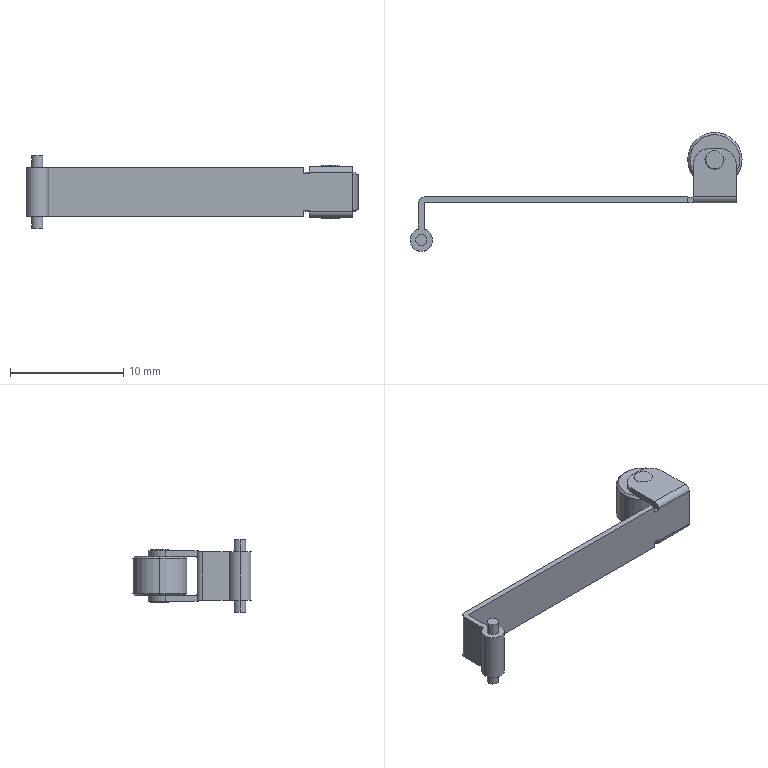Part | SolidWorks | features ICE 5, Fillet 3, Chamfer 2, Extrusion 1 | 3 solids | 53 faces | box 29.3 x 10.5 x 6.4 mm | volume 172.618 mm3 | plane 25 | cylinder 20 | cone 8 | commonest cylinder face diameters 1 x7 2 x5 3 x4 0.4 x2 4.8 x2
STEP:
#1=CARTESIAN_POINT('',(0.5,0.,3.2));
#2=VERTEX_POINT('',#1);
#3=CARTESIAN_POINT('',(-0.5,0.,3.2));
#4=VERTEX_POINT('',#3);
#5=CARTESIAN_POINT('',(0.,0.,3.2));
#6=DIRECTION('',(0.,0.,1.));
#7=DIRECTION('',(1.,0.,0.));
#8=AXIS2_PLACEMENT_3D('',#5,#6,#7);
#9=CIRCLE('',#8,0.5);
#10=EDGE_CURVE('',#2,#4,#9,.T.);
#11=ORIENTED_EDGE('',*,*,#10,.F.);
#12=CARTESIAN_POINT('',(0.5,0.,2.15));
#13=VERTEX_POINT('',#12);
#14=CARTESIAN_POINT('',(0.5,0.,3.2));
#15=DIRECTION('',(0.,0.,-1.));
#16=VECTOR('',#15,1000.);
#17=LINE('',#14,#16);
#18=EDGE_CURVE('',#2,#13,#17,.T.);
#19=ORIENTED_EDGE('',*,*,#18,.T.);
#20=CARTESIAN_POINT('',(-0.5,0.,2.15));
#21=VERTEX_POINT('',#20);
#22=CARTESIAN_POINT('',(0.,0.,2.15));
#23=DIRECTION('',(0.,0.,1.));
#24=DIRECTION('',(1.,0.,0.));
#25=AXIS2_PLACEMENT_3D('',#22,#23,#24);
#26=CIRCLE('',#25,0.5);
#27=EDGE_CURVE('',#13,#21,#26,.T.);
#28=ORIENTED_EDGE('',*,*,#27,.T.);
#29=CARTESIAN_POINT('',(-0.5,0.,3.2));
#30=DIRECTION('',(0.,0.,-1.));
#31=VECTOR('',#30,1000.);
#32=LINE('',#29,#31);
#33=EDGE_CURVE('',#4,#21,#32,.T.);
#34=ORIENTED_EDGE('',*,*,#33,.F.);
#35=EDGE_LOOP('',(#11,#19,#28,#34));
#36=FACE_OUTER_BOUND('',#35,.T.);
#37=CARTESIAN_POINT('',(0.,0.,3.2));
#38=DIRECTION('',(0.,0.,-1.));
#39=DIRECTION('',(-1.,0.,0.));
#40=AXIS2_PLACEMENT_3D('',#37,#38,#39);
#41=CYLINDRICAL_SURFACE('',#40,0.5);
#42=ADVANCED_FACE('',(#36),#41,.T.);
#43=CARTESIAN_POINT('',(-0.5,0.,-2.15));
#44=VERTEX_POINT('',#43);
#45=CARTESIAN_POINT('',(0.5,0.,-2.15));
#46=VERTEX_POINT('',#45);
#47=CARTESIAN_POINT('',(0.,0.,-2.15));
#48=DIRECTION('',(0.,0.,-1.));
#49=DIRECTION('',(1.,0.,0.));
#50=AXIS2_PLACEMENT_3D('',#47,#48,#49);
#51=CIRCLE('',#50,0.5);
#52=EDGE_CURVE('',#44,#46,#51,.T.);
#53=ORIENTED_EDGE('',*,*,#52,.T.);
#54=CARTESIAN_POINT('',(0.5,0.,-3.2));
#55=VERTEX_POINT('',#54);
#56=CARTESIAN_POINT('',(0.5,0.,3.2));
#57=DIRECTION('',(0.,0.,-1.));
#58=VECTOR('',#57,1000.);
#59=LINE('',#56,#58);
#60=EDGE_CURVE('',#46,#55,#59,.T.);
#61=ORIENTED_EDGE('',*,*,#60,.T.);
#62=CARTESIAN_POINT('',(-0.5,0.,-3.2));
#63=VERTEX_POINT('',#62);
#64=CARTESIAN_POINT('',(0.,0.,-3.2));
#65=DIRECTION('',(0.,0.,1.));
#66=DIRECTION('',(1.,0.,0.));
#67=AXIS2_PLACEMENT_3D('',#64,#65,#66);
#68=CIRCLE('',#67,0.5);
#69=EDGE_CURVE('',#55,#63,#68,.T.);
#70=ORIENTED_EDGE('',*,*,#69,.T.);
#71=CARTESIAN_POINT('',(-0.5,0.,3.2));
#72=DIRECTION('',(0.,0.,-1.));
#73=VECTOR('',#72,1000.);
#74=LINE('',#71,#73);
#75=EDGE_CURVE('',#44,#63,#74,.T.);
#76=ORIENTED_EDGE('',*,*,#75,.F.);
#77=EDGE_LOOP('',(#53,#61,#70,#76));
#78=FACE_OUTER_BOUND('',#77,.T.);
#79=CARTESIAN_POINT('',(0.,0.,3.2));
#80=DIRECTION('',(0.,0.,-1.));
#81=DIRECTION('',(-1.,0.,0.));
#82=AXIS2_PLACEMENT_3D('',#79,#80,#81);
#83=CYLINDRICAL_SURFACE('',#82,0.5);
#84=ADVANCED_FACE('',(#78),#83,.T.);
#85=CARTESIAN_POINT('',(1.,0.,2.15));
#86=VERTEX_POINT('',#85);
#87=CARTESIAN_POINT('',(0.25,0.9682,2.15));
#88=VERTEX_POINT('',#87);
#89=CARTESIAN_POINT('',(0.,0.,2.15));
#90=DIRECTION('',(0.,0.,1.));
#91=DIRECTION('',(1.,0.,0.));
#92=AXIS2_PLACEMENT_3D('',#89,#90,#91);
#93=CIRCLE('',#92,1.);
#94=EDGE_CURVE('',#86,#88,#93,.T.);
#95=ORIENTED_EDGE('',*,*,#94,.F.);
#96=CARTESIAN_POINT('',(1.,0.,-2.15));
#97=VERTEX_POINT('',#96);
#98=CARTESIAN_POINT('',(1.,0.,2.15));
#99=DIRECTION('',(0.,0.,-1.));
#100=VECTOR('',#99,1000.);
#101=LINE('',#98,#100);
#102=EDGE_CURVE('',#86,#97,#101,.T.);
#103=ORIENTED_EDGE('',*,*,#102,.T.);
#104=CARTESIAN_POINT('',(0.25,0.9682,-2.15));
#105=VERTEX_POINT('',#104);
#106=CARTESIAN_POINT('',(0.,0.,-2.15));
#107=DIRECTION('',(0.,0.,1.));
#108=DIRECTION('',(1.,0.,0.));
#109=AXIS2_PLACEMENT_3D('',#106,#107,#108);
#110=CIRCLE('',#109,1.);
#111=EDGE_CURVE('',#97,#105,#110,.T.);
#112=ORIENTED_EDGE('',*,*,#111,.T.);
#113=CARTESIAN_POINT('',(0.25,0.9682,2.15));
#114=DIRECTION('',(0.,0.,-1.));
#115=VECTOR('',#114,1000.);
#116=LINE('',#113,#115);
#117=EDGE_CURVE('',#88,#105,#116,.T.);
#118=ORIENTED_EDGE('',*,*,#117,.F.);
#119=EDGE_LOOP('',(#95,#103,#112,#118));
#120=FACE_OUTER_BOUND('',#119,.T.);
#121=CARTESIAN_POINT('',(0.,0.,2.15));
#122=DIRECTION('',(0.,0.,-1.));
#123=DIRECTION('',(-1.,0.,0.));
#124=AXIS2_PLACEMENT_3D('',#121,#122,#123);
#125=CYLINDRICAL_SURFACE('',#124,1.);
#126=ADVANCED_FACE('',(#120),#125,.T.);
#127=ORIENTED_EDGE('',*,*,#102,.F.);
#128=CARTESIAN_POINT('',(-1.,0.,2.15));
#129=VERTEX_POINT('',#128);
#130=CARTESIAN_POINT('',(0.,0.,2.15));
#131=DIRECTION('',(0.,0.,1.));
#132=DIRECTION('',(1.,0.,0.));
#133=AXIS2_PLACEMENT_3D('',#130,#131,#132);
#134=CIRCLE('',#133,1.);
#135=EDGE_CURVE('',#129,#86,#134,.T.);
#136=ORIENTED_EDGE('',*,*,#135,.F.);
#137=CARTESIAN_POINT('',(-1.,0.,-2.15));
#138=VERTEX_POINT('',#137);
#139=CARTESIAN_POINT('',(-1.,0.,2.15));
#140=DIRECTION('',(0.,0.,-1.));
#141=VECTOR('',#140,1000.);
#142=LINE('',#139,#141);
#143=EDGE_CURVE('',#129,#138,#142,.T.);
#144=ORIENTED_EDGE('',*,*,#143,.T.);
#145=CARTESIAN_POINT('',(0.,0.,-2.15));
#146=DIRECTION('',(0.,0.,1.));
#147=DIRECTION('',(1.,0.,0.));
#148=AXIS2_PLACEMENT_3D('',#145,#146,#147);
#149=CIRCLE('',#148,1.);
#150=EDGE_CURVE('',#138,#97,#149,.T.);
#151=ORIENTED_EDGE('',*,*,#150,.T.);
#152=EDGE_LOOP('',(#127,#136,#144,#151));
#153=FACE_OUTER_BOUND('',#152,.T.);
#154=CARTESIAN_POINT('',(0.,0.,2.15));
#155=DIRECTION('',(0.,0.,-1.));
#156=DIRECTION('',(-1.,0.,0.));
#157=AXIS2_PLACEMENT_3D('',#154,#155,#156);
#158=CYLINDRICAL_SURFACE('',#157,1.);
#159=ADVANCED_FACE('',(#153),#158,.T.);
#160=ORIENTED_EDGE('',*,*,#52,.F.);
#161=CARTESIAN_POINT('',(0.,0.,-2.15));
#162=DIRECTION('',(0.,0.,-1.));
#163=DIRECTION('',(1.,0.,0.));
#164=AXIS2_PLACEMENT_3D('',#161,#162,#163);
#165=CIRCLE('',#164,0.5);
#166=EDGE_CURVE('',#46,#44,#165,.T.);
#167=ORIENTED_EDGE('',*,*,#166,.F.);
#168=EDGE_LOOP('',(#160,#167));
#169=FACE_BOUND('',#168,.T.);
#170=CARTESIAN_POINT('',(23.5,3.8,-2.15));
#171=VERTEX_POINT('',#170);
#172=CARTESIAN_POINT('',(0.25,3.8,-2.15));
#173=VERTEX_POINT('',#172);
#174=CARTESIAN_POINT('',(0.25,3.8,-2.15));
#175=DIRECTION('',(-1.,0.,0.));
#176=VECTOR('',#175,1000.);
#177=LINE('',#174,#176);
#178=EDGE_CURVE('',#171,#173,#177,.T.);
#179=ORIENTED_EDGE('',*,*,#178,.F.);
#180=CARTESIAN_POINT('',(23.5,3.3,-2.15));
#181=VERTEX_POINT('',#180);
#182=CARTESIAN_POINT('',(23.5,0.,-2.15));
#183=DIRECTION('',(0.,-1.,0.));
#184=VECTOR('',#183,1000.);
#185=LINE('',#182,#184);
#186=EDGE_CURVE('',#171,#181,#185,.T.);
#187=ORIENTED_EDGE('',*,*,#186,.T.);
#188=CARTESIAN_POINT('',(0.25,3.3,-2.15));
#189=VERTEX_POINT('',#188);
#190=CARTESIAN_POINT('',(0.25,3.3,-2.15));
#191=DIRECTION('',(1.,0.,0.));
#192=VECTOR('',#191,1000.);
#193=LINE('',#190,#192);
#194=EDGE_CURVE('',#189,#181,#193,.T.);
#195=ORIENTED_EDGE('',*,*,#194,.F.);
#196=CARTESIAN_POINT('',(0.25,3.3,-2.15));
#197=DIRECTION('',(0.,1.,0.));
#198=VECTOR('',#197,1000.);
#199=LINE('',#196,#198);
#200=EDGE_CURVE('',#105,#189,#199,.T.);
#201=ORIENTED_EDGE('',*,*,#200,.F.);
#202=ORIENTED_EDGE('',*,*,#111,.F.);
#203=ORIENTED_EDGE('',*,*,#150,.F.);
#204=CARTESIAN_POINT('',(-0.25,0.9682,-2.15));
#205=VERTEX_POINT('',#204);
#206=CARTESIAN_POINT('',(0.,0.,-2.15));
#207=DIRECTION('',(0.,0.,1.));
#208=DIRECTION('',(1.,0.,0.));
#209=AXIS2_PLACEMENT_3D('',#206,#207,#208);
#210=CIRCLE('',#209,1.);
#211=EDGE_CURVE('',#205,#138,#210,.T.);
#212=ORIENTED_EDGE('',*,*,#211,.F.);
#213=CARTESIAN_POINT('',(-0.25,3.3,-2.15));
#214=VERTEX_POINT('',#213);
#215=CARTESIAN_POINT('',(-0.25,3.3,-2.15));
#216=DIRECTION('',(0.,-1.,0.));
#217=VECTOR('',#216,1000.);
#218=LINE('',#215,#217);
#219=EDGE_CURVE('',#214,#205,#218,.T.);
#220=ORIENTED_EDGE('',*,*,#219,.F.);
#221=CARTESIAN_POINT('',(0.25,3.3,-2.15));
#222=DIRECTION('',(0.,0.,1.));
#223=DIRECTION('',(-1.,0.,0.));
#224=AXIS2_PLACEMENT_3D('',#221,#222,#223);
#225=CIRCLE('',#224,0.5);
#226=EDGE_CURVE('',#173,#214,#225,.T.);
#227=ORIENTED_EDGE('',*,*,#226,.F.);
#228=EDGE_LOOP('',(#179,#187,#195,#201,#202,#203,#212,#220,#227));
#229=FACE_OUTER_BOUND('',#228,.T.);
#230=CARTESIAN_POINT('',(0.,0.,-2.15));
#231=DIRECTION('',(0.,0.,1.));
#232=DIRECTION('',(1.,0.,0.));
#233=AXIS2_PLACEMENT_3D('',#230,#231,#232);
#234=PLANE('',#233);
#235=ADVANCED_FACE('',(#169,#229),#234,.F.);
#236=CARTESIAN_POINT('',(23.5,3.8,2.15));
#237=VERTEX_POINT('',#236);
#238=CARTESIAN_POINT('',(23.5,3.3,2.15));
#239=VERTEX_POINT('',#238);
#240=CARTESIAN_POINT('',(23.5,0.,2.15));
#241=DIRECTION('',(0.,-1.,0.));
#242=VECTOR('',#241,1000.);
#243=LINE('',#240,#242);
#244=EDGE_CURVE('',#237,#239,#243,.T.);
#245=ORIENTED_EDGE('',*,*,#244,.F.);
#246=CARTESIAN_POINT('',(0.25,3.8,2.15));
#247=VERTEX_POINT('',#246);
#248=CARTESIAN_POINT('',(0.25,3.8,2.15));
#249=DIRECTION('',(-1.,0.,0.));
#250=VECTOR('',#249,1000.);
#251=LINE('',#248,#250);
#252=EDGE_CURVE('',#237,#247,#251,.T.);
#253=ORIENTED_EDGE('',*,*,#252,.T.);
#254=CARTESIAN_POINT('',(-0.25,3.3,2.15));
#255=VERTEX_POINT('',#254);
#256=CARTESIAN_POINT('',(0.25,3.3,2.15));
#257=DIRECTION('',(0.,0.,1.));
#258=DIRECTION('',(-1.,0.,0.));
#259=AXIS2_PLACEMENT_3D('',#256,#257,#258);
#260=CIRCLE('',#259,0.5);
#261=EDGE_CURVE('',#247,#255,#260,.T.);
#262=ORIENTED_EDGE('',*,*,#261,.T.);
#263=CARTESIAN_POINT('',(-0.25,0.9682,2.15));
#264=VERTEX_POINT('',#263);
#265=CARTESIAN_POINT('',(-0.25,3.3,2.15));
#266=DIRECTION('',(0.,-1.,0.));
#267=VECTOR('',#266,1000.);
#268=LINE('',#265,#267);
#269=EDGE_CURVE('',#255,#264,#268,.T.);
#270=ORIENTED_EDGE('',*,*,#269,.T.);
#271=CARTESIAN_POINT('',(0.,0.,2.15));
#272=DIRECTION('',(0.,0.,1.));
#273=DIRECTION('',(1.,0.,0.));
#274=AXIS2_PLACEMENT_3D('',#271,#272,#273);
#275=CIRCLE('',#274,1.);
#276=EDGE_CURVE('',#264,#129,#275,.T.);
#277=ORIENTED_EDGE('',*,*,#276,.T.);
#278=ORIENTED_EDGE('',*,*,#135,.T.);
#279=ORIENTED_EDGE('',*,*,#94,.T.);
#280=CARTESIAN_POINT('',(0.25,3.3,2.15));
#281=VERTEX_POINT('',#280);
#282=CARTESIAN_POINT('',(0.25,3.3,2.15));
#283=DIRECTION('',(0.,1.,0.));
#284=VECTOR('',#283,1000.);
#285=LINE('',#282,#284);
#286=EDGE_CURVE('',#88,#281,#285,.T.);
#287=ORIENTED_EDGE('',*,*,#286,.T.);
#288=CARTESIAN_POINT('',(0.25,3.3,2.15));
#289=DIRECTION('',(1.,0.,0.));
#290=VECTOR('',#289,1000.);
#291=LINE('',#288,#290);
#292=EDGE_CURVE('',#281,#239,#291,.T.);
#293=ORIENTED_EDGE('',*,*,#292,.T.);
#294=EDGE_LOOP('',(#245,#253,#262,#270,#277,#278,#279,#287,#293));
#295=FACE_OUTER_BOUND('',#294,.T.);
#296=CARTESIAN_POINT('',(0.,0.,2.15));
#297=DIRECTION('',(0.,0.,1.));
#298=DIRECTION('',(1.,0.,0.));
#299=AXIS2_PLACEMENT_3D('',#296,#297,#298);
#300=CIRCLE('',#299,0.5);
#301=EDGE_CURVE('',#21,#13,#300,.T.);
#302=ORIENTED_EDGE('',*,*,#301,.F.);
#303=ORIENTED_EDGE('',*,*,#27,.F.);
#304=EDGE_LOOP('',(#302,#303));
#305=FACE_BOUND('',#304,.T.);
#306=CARTESIAN_POINT('',(0.,0.,2.15));
#307=DIRECTION('',(0.,0.,1.));
#308=DIRECTION('',(1.,0.,0.));
#309=AXIS2_PLACEMENT_3D('',#306,#307,#308);
#310=PLANE('',#309);
#311=ADVANCED_FACE('',(#295,#305),#310,.T.);
#312=ORIENTED_EDGE('',*,*,#143,.F.);
#313=ORIENTED_EDGE('',*,*,#276,.F.);
#314=CARTESIAN_POINT('',(-0.25,0.9682,2.15));
#315=DIRECTION('',(0.,0.,-1.));
#316=VECTOR('',#315,1000.);
#317=LINE('',#314,#316);
#318=EDGE_CURVE('',#264,#205,#317,.T.);
#319=ORIENTED_EDGE('',*,*,#318,.T.);
#320=ORIENTED_EDGE('',*,*,#211,.T.);
#321=EDGE_LOOP('',(#312,#313,#319,#320));
#322=FACE_OUTER_BOUND('',#321,.T.);
#323=CARTESIAN_POINT('',(0.,0.,2.15));
#324=DIRECTION('',(0.,0.,-1.));
#325=DIRECTION('',(-1.,0.,0.));
#326=AXIS2_PLACEMENT_3D('',#323,#324,#325);
#327=CYLINDRICAL_SURFACE('',#326,1.);
#328=ADVANCED_FACE('',(#322),#327,.T.);
#329=ORIENTED_EDGE('',*,*,#200,.T.);
#330=CARTESIAN_POINT('',(0.25,3.3,2.15));
#331=DIRECTION('',(0.,0.,-1.));
#332=VECTOR('',#331,1000.);
#333=LINE('',#330,#332);
#334=EDGE_CURVE('',#281,#189,#333,.T.);
#335=ORIENTED_EDGE('',*,*,#334,.F.);
#336=ORIENTED_EDGE('',*,*,#286,.F.);
#337=ORIENTED_EDGE('',*,*,#117,.T.);
#338=EDGE_LOOP('',(#329,#335,#336,#337));
#339=FACE_OUTER_BOUND('',#338,.T.);
#340=CARTESIAN_POINT('',(0.25,3.3,2.15));
#341=DIRECTION('',(-1.,0.,0.));
#342=DIRECTION('',(0.,-1.,0.));
#343=AXIS2_PLACEMENT_3D('',#340,#341,#342);
#344=PLANE('',#343);
#345=ADVANCED_FACE('',(#339),#344,.F.);
#346=CARTESIAN_POINT('',(27.8,3.3,1.75));
#347=VERTEX_POINT('',#346);
#348=CARTESIAN_POINT('',(27.8,3.3,-1.75));
#349=VERTEX_POINT('',#348);
#350=CARTESIAN_POINT('',(27.8,3.3,2.15));
#351=DIRECTION('',(0.,0.,-1.));
#352=VECTOR('',#351,1000.);
#353=LINE('',#350,#352);
#354=EDGE_CURVE('',#347,#349,#353,.T.);
#355=ORIENTED_EDGE('',*,*,#354,.F.);
#356=CARTESIAN_POINT('',(24.,3.3,1.75));
#357=VERTEX_POINT('',#356);
#358=CARTESIAN_POINT('',(24.,3.3,1.75));
#359=DIRECTION('',(-1.,0.,0.));
#360=VECTOR('',#359,1000.);
#361=LINE('',#358,#360);
#362=EDGE_CURVE('',#347,#357,#361,.T.);
#363=ORIENTED_EDGE('',*,*,#362,.T.);
#364=CARTESIAN_POINT('',(24.,3.3,1.6));
#365=VERTEX_POINT('',#364);
#366=CARTESIAN_POINT('',(24.,3.3,2.15));
#367=DIRECTION('',(0.,0.,-1.));
#368=VECTOR('',#367,1000.);
#369=LINE('',#366,#368);
#370=EDGE_CURVE('',#357,#365,#369,.T.);
#371=ORIENTED_EDGE('',*,*,#370,.T.);
#372=CARTESIAN_POINT('',(23.5,3.3,1.6));
#373=VERTEX_POINT('',#372);
#374=CARTESIAN_POINT('',(0.25,3.3,1.6));
#375=DIRECTION('',(-1.,0.,0.));
#376=VECTOR('',#375,1000.);
#377=LINE('',#374,#376);
#378=EDGE_CURVE('',#365,#373,#377,.T.);
#379=ORIENTED_EDGE('',*,*,#378,.T.);
#380=CARTESIAN_POINT('',(23.5,3.3,2.15));
#381=DIRECTION('',(0.,0.,1.));
#382=VECTOR('',#381,1000.);
#383=LINE('',#380,#382);
#384=EDGE_CURVE('',#373,#239,#383,.T.);
#385=ORIENTED_EDGE('',*,*,#384,.T.);
#386=ORIENTED_EDGE('',*,*,#292,.F.);
#387=ORIENTED_EDGE('',*,*,#334,.T.);
#388=ORIENTED_EDGE('',*,*,#194,.T.);
#389=CARTESIAN_POINT('',(23.5,3.3,-1.6));
#390=VERTEX_POINT('',#389);
#391=CARTESIAN_POINT('',(23.5,3.3,2.15));
#392=DIRECTION('',(0.,0.,1.));
#393=VECTOR('',#392,1000.);
#394=LINE('',#391,#393);
#395=EDGE_CURVE('',#181,#390,#394,.T.);
#396=ORIENTED_EDGE('',*,*,#395,.T.);
#397=CARTESIAN_POINT('',(24.,3.3,-1.6));
#398=VERTEX_POINT('',#397);
#399=CARTESIAN_POINT('',(0.25,3.3,-1.6));
#400=DIRECTION('',(1.,0.,0.));
#401=VECTOR('',#400,1000.);
#402=LINE('',#399,#401);
#403=EDGE_CURVE('',#390,#398,#402,.T.);
#404=ORIENTED_EDGE('',*,*,#403,.T.);
#405=CARTESIAN_POINT('',(24.,3.3,-1.75));
#406=VERTEX_POINT('',#405);
#407=CARTESIAN_POINT('',(24.,3.3,-2.15));
#408=DIRECTION('',(0.,0.,-1.));
#409=VECTOR('',#408,1000.);
#410=LINE('',#407,#409);
#411=EDGE_CURVE('',#398,#406,#410,.T.);
#412=ORIENTED_EDGE('',*,*,#411,.T.);
#413=CARTESIAN_POINT('',(27.8,3.3,-1.75));
#414=DIRECTION('',(1.,0.,0.));
#415=VECTOR('',#414,1000.);
#416=LINE('',#413,#415);
#417=EDGE_CURVE('',#406,#349,#416,.T.);
#418=ORIENTED_EDGE('',*,*,#417,.T.);
#419=EDGE_LOOP('',(#355,#363,#371,#379,#385,#386,#387,#388,#396,#404,#412,#418));
#420=FACE_OUTER_BOUND('',#419,.T.);
#421=CARTESIAN_POINT('',(0.25,3.3,2.15));
#422=DIRECTION('',(0.,1.,0.));
#423=DIRECTION('',(0.,0.,1.));
#424=AXIS2_PLACEMENT_3D('',#421,#422,#423);
#425=PLANE('',#424);
#426=ADVANCED_FACE('',(#420),#425,.F.);
#427=CARTESIAN_POINT('',(27.8,3.8,-2.25));
#428=VERTEX_POINT('',#427);
#429=CARTESIAN_POINT('',(27.8,6.6,-2.25));
#430=VERTEX_POINT('',#429);
#431=CARTESIAN_POINT('',(27.8,3.3,-2.25));
#432=DIRECTION('',(0.,1.,0.));
#433=VECTOR('',#432,1000.);
#434=LINE('',#431,#433);
#435=EDGE_CURVE('',#428,#430,#434,.T.);
#436=ORIENTED_EDGE('',*,*,#435,.T.);
#437=CARTESIAN_POINT('',(27.8,6.6,-1.75));
#438=VERTEX_POINT('',#437);
#439=CARTESIAN_POINT('',(27.8,6.6,-1.75));
#440=DIRECTION('',(0.,0.,1.));
#441=VECTOR('',#440,1000.);
#442=LINE('',#439,#441);
#443=EDGE_CURVE('',#430,#438,#442,.T.);
#444=ORIENTED_EDGE('',*,*,#443,.T.);
#445=CARTESIAN_POINT('',(27.8,4.,-1.75));
#446=VERTEX_POINT('',#445);
#447=CARTESIAN_POINT('',(27.8,3.8,-1.75));
#448=DIRECTION('',(0.,-1.,0.));
#449=VECTOR('',#448,1000.);
#450=LINE('',#447,#449);
#451=EDGE_CURVE('',#438,#446,#450,.T.);
#452=ORIENTED_EDGE('',*,*,#451,.T.);
#453=CARTESIAN_POINT('',(27.8,3.8,-1.55));
#454=VERTEX_POINT('',#453);
#455=CARTESIAN_POINT('',(27.8,4.,-1.55));
#456=DIRECTION('',(-1.,0.,0.));
#457=DIRECTION('',(0.,0.,1.));
#458=AXIS2_PLACEMENT_3D('',#455,#456,#457);
#459=CIRCLE('',#458,0.2);
#460=EDGE_CURVE('',#446,#454,#459,.T.);
#461=ORIENTED_EDGE('',*,*,#460,.T.);
#462=CARTESIAN_POINT('',(27.8,3.8,1.55));
#463=VERTEX_POINT('',#462);
#464=CARTESIAN_POINT('',(27.8,3.8,2.15));
#465=DIRECTION('',(0.,0.,-1.));
#466=VECTOR('',#465,1000.);
#467=LINE('',#464,#466);
#468=EDGE_CURVE('',#463,#454,#467,.T.);
#469=ORIENTED_EDGE('',*,*,#468,.F.);
#470=CARTESIAN_POINT('',(27.8,4.,1.75));
#471=VERTEX_POINT('',#470);
#472=CARTESIAN_POINT('',(27.8,4.,1.55));
#473=DIRECTION('',(-1.,0.,0.));
#474=DIRECTION('',(0.,0.,1.));
#475=AXIS2_PLACEMENT_3D('',#472,#473,#474);
#476=CIRCLE('',#475,0.2);
#477=EDGE_CURVE('',#463,#471,#476,.T.);
#478=ORIENTED_EDGE('',*,*,#477,.T.);
#479=CARTESIAN_POINT('',(27.8,6.6,1.75));
#480=VERTEX_POINT('',#479);
#481=CARTESIAN_POINT('',(27.8,3.8,1.75));
#482=DIRECTION('',(0.,1.,0.));
#483=VECTOR('',#482,1000.);
#484=LINE('',#481,#483);
#485=EDGE_CURVE('',#471,#480,#484,.T.);
#486=ORIENTED_EDGE('',*,*,#485,.T.);
#487=CARTESIAN_POINT('',(27.8,6.6,2.25));
#488=VERTEX_POINT('',#487);
#489=CARTESIAN_POINT('',(27.8,6.6,2.25));
#490=DIRECTION('',(0.,0.,1.));
#491=VECTOR('',#490,1000.);
#492=LINE('',#489,#491);
#493=EDGE_CURVE('',#480,#488,#492,.T.);
#494=ORIENTED_EDGE('',*,*,#493,.T.);
#495=CARTESIAN_POINT('',(27.8,3.8,2.25));
#496=VERTEX_POINT('',#495);
#497=CARTESIAN_POINT('',(27.8,3.3,2.25));
#498=DIRECTION('',(0.,-1.,0.));
#499=VECTOR('',#498,1000.);
#500=LINE('',#497,#499);
#501=EDGE_CURVE('',#488,#496,#500,.T.);
#502=ORIENTED_EDGE('',*,*,#501,.T.);
#503=CARTESIAN_POINT('',(27.8,3.8,1.75));
#504=DIRECTION('',(1.,0.,0.));
#505=DIRECTION('',(0.,0.,1.));
#506=AXIS2_PLACEMENT_3D('',#503,#504,#505);
#507=CIRCLE('',#506,0.5);
#508=EDGE_CURVE('',#496,#347,#507,.T.);
#509=ORIENTED_EDGE('',*,*,#508,.T.);
#510=ORIENTED_EDGE('',*,*,#354,.T.);
#511=CARTESIAN_POINT('',(27.8,3.8,-1.75));
#512=DIRECTION('',(1.,0.,0.));
#513=DIRECTION('',(0.,0.,1.));
#514=AXIS2_PLACEMENT_3D('',#511,#512,#513);
#515=CIRCLE('',#514,0.5);
#516=EDGE_CURVE('',#349,#428,#515,.T.);
#517=ORIENTED_EDGE('',*,*,#516,.T.);
#518=EDGE_LOOP('',(#436,#444,#452,#461,#469,#478,#486,#494,#502,#509,#510,#517));
#519=FACE_OUTER_BOUND('',#518,.T.);
#520=CARTESIAN_POINT('',(27.8,3.8,2.15));
#521=DIRECTION('',(-1.,0.,0.));
#522=DIRECTION('',(0.,0.,1.));
#523=AXIS2_PLACEMENT_3D('',#520,#521,#522);
#524=PLANE('',#523);
#525=ADVANCED_FACE('',(#519),#524,.F.);
#526=ORIENTED_EDGE('',*,*,#252,.F.);
#527=CARTESIAN_POINT('',(23.5,3.8,1.6));
#528=VERTEX_POINT('',#527);
#529=CARTESIAN_POINT('',(23.5,3.8,2.25));
#530=DIRECTION('',(0.,0.,1.));
#531=VECTOR('',#530,1000.);
#532=LINE('',#529,#531);
#533=EDGE_CURVE('',#528,#237,#532,.T.);
#534=ORIENTED_EDGE('',*,*,#533,.F.);
#535=CARTESIAN_POINT('',(24.,3.8,1.6));
#536=VERTEX_POINT('',#535);
#537=CARTESIAN_POINT('',(24.,3.8,1.6));
#538=DIRECTION('',(-1.,0.,0.));
#539=VECTOR('',#538,1000.);
#540=LINE('',#537,#539);
#541=EDGE_CURVE('',#536,#528,#540,.T.);
#542=ORIENTED_EDGE('',*,*,#541,.F.);
#543=CARTESIAN_POINT('',(24.,3.8,1.55));
#544=VERTEX_POINT('',#543);
#545=CARTESIAN_POINT('',(24.,3.8,2.15));
#546=DIRECTION('',(0.,0.,-1.));
#547=VECTOR('',#546,1000.);
#548=LINE('',#545,#547);
#549=EDGE_CURVE('',#536,#544,#548,.T.);
#550=ORIENTED_EDGE('',*,*,#549,.T.);
#551=CARTESIAN_POINT('',(0.25,3.8,1.55));
#552=DIRECTION('',(1.,0.,0.));
#553=VECTOR('',#552,1000.);
#554=LINE('',#551,#553);
#555=EDGE_CURVE('',#544,#463,#554,.T.);
#556=ORIENTED_EDGE('',*,*,#555,.T.);
#557=ORIENTED_EDGE('',*,*,#468,.T.);
#558=CARTESIAN_POINT('',(24.,3.8,-1.55));
#559=VERTEX_POINT('',#558);
#560=CARTESIAN_POINT('',(0.25,3.8,-1.55));
#561=DIRECTION('',(-1.,0.,0.));
#562=VECTOR('',#561,1000.);
#563=LINE('',#560,#562);
#564=EDGE_CURVE('',#454,#559,#563,.T.);
#565=ORIENTED_EDGE('',*,*,#564,.T.);
#566=CARTESIAN_POINT('',(24.,3.8,-1.6));
#567=VERTEX_POINT('',#566);
#568=CARTESIAN_POINT('',(24.,3.8,-2.15));
#569=DIRECTION('',(0.,0.,-1.));
#570=VECTOR('',#569,1000.);
#571=LINE('',#568,#570);
#572=EDGE_CURVE('',#559,#567,#571,.T.);
#573=ORIENTED_EDGE('',*,*,#572,.T.);
#574=CARTESIAN_POINT('',(23.5,3.8,-1.6));
#575=VERTEX_POINT('',#574);
#576=CARTESIAN_POINT('',(24.,3.8,-1.6));
#577=DIRECTION('',(1.,0.,0.));
#578=VECTOR('',#577,1000.);
#579=LINE('',#576,#578);
#580=EDGE_CURVE('',#575,#567,#579,.T.);
#581=ORIENTED_EDGE('',*,*,#580,.F.);
#582=CARTESIAN_POINT('',(23.5,3.8,-2.25));
#583=DIRECTION('',(0.,0.,1.));
#584=VECTOR('',#583,1000.);
#585=LINE('',#582,#584);
#586=EDGE_CURVE('',#171,#575,#585,.T.);
#587=ORIENTED_EDGE('',*,*,#586,.F.);
#588=ORIENTED_EDGE('',*,*,#178,.T.);
#589=CARTESIAN_POINT('',(0.25,3.8,2.15));
#590=DIRECTION('',(0.,0.,-1.));
#591=VECTOR('',#590,1000.);
#592=LINE('',#589,#591);
#593=EDGE_CURVE('',#247,#173,#592,.T.);
#594=ORIENTED_EDGE('',*,*,#593,.F.);
#595=EDGE_LOOP('',(#526,#534,#542,#550,#556,#557,#565,#573,#581,#587,#588,#594));
#596=FACE_OUTER_BOUND('',#595,.T.);
#597=CARTESIAN_POINT('',(0.25,3.8,2.15));
#598=DIRECTION('',(0.,-1.,0.));
#599=DIRECTION('',(1.,0.,0.));
#600=AXIS2_PLACEMENT_3D('',#597,#598,#599);
#601=PLANE('',#600);
#602=ADVANCED_FACE('',(#596),#601,.F.);
#603=ORIENTED_EDGE('',*,*,#226,.T.);
#604=CARTESIAN_POINT('',(-0.25,3.3,2.15));
#605=DIRECTION('',(0.,0.,-1.));
#606=VECTOR('',#605,1000.);
#607=LINE('',#604,#606);
#608=EDGE_CURVE('',#255,#214,#607,.T.);
#609=ORIENTED_EDGE('',*,*,#608,.F.);
#610=ORIENTED_EDGE('',*,*,#261,.F.);
#611=ORIENTED_EDGE('',*,*,#593,.T.);
#612=EDGE_LOOP('',(#603,#609,#610,#611));
#613=FACE_OUTER_BOUND('',#612,.T.);
#614=CARTESIAN_POINT('',(0.25,3.3,2.15));
#615=DIRECTION('',(0.,0.,-1.));
#616=DIRECTION('',(-1.,0.,0.));
#617=AXIS2_PLACEMENT_3D('',#614,#615,#616);
#618=CYLINDRICAL_SURFACE('',#617,0.5);
#619=ADVANCED_FACE('',(#613),#618,.T.);
#620=ORIENTED_EDGE('',*,*,#219,.T.);
#621=ORIENTED_EDGE('',*,*,#318,.F.);
#622=ORIENTED_EDGE('',*,*,#269,.F.);
#623=ORIENTED_EDGE('',*,*,#608,.T.);
#624=EDGE_LOOP('',(#620,#621,#622,#623));
#625=FACE_OUTER_BOUND('',#624,.T.);
#626=CARTESIAN_POINT('',(-0.25,3.3,2.15));
#627=DIRECTION('',(1.,0.,0.));
#628=DIRECTION('',(0.,1.,0.));
#629=AXIS2_PLACEMENT_3D('',#626,#627,#628);
#630=PLANE('',#629);
#631=ADVANCED_FACE('',(#625),#630,.F.);
#632=CARTESIAN_POINT('',(0.,0.,-3.2));
#633=DIRECTION('',(0.,0.,1.));
#634=DIRECTION('',(1.,0.,0.));
#635=AXIS2_PLACEMENT_3D('',#632,#633,#634);
#636=CIRCLE('',#635,0.5);
#637=EDGE_CURVE('',#63,#55,#636,.T.);
#638=ORIENTED_EDGE('',*,*,#637,.F.);
#639=ORIENTED_EDGE('',*,*,#69,.F.);
#640=EDGE_LOOP('',(#638,#639));
#641=FACE_OUTER_BOUND('',#640,.T.);
#642=CARTESIAN_POINT('',(0.,0.,-3.2));
#643=DIRECTION('',(0.,0.,1.));
#644=DIRECTION('',(1.,0.,0.));
#645=AXIS2_PLACEMENT_3D('',#642,#643,#644);
#646=PLANE('',#645);
#647=ADVANCED_FACE('',(#641),#646,.F.);
#648=ORIENTED_EDGE('',*,*,#60,.F.);
#649=ORIENTED_EDGE('',*,*,#166,.T.);
#650=ORIENTED_EDGE('',*,*,#75,.T.);
#651=ORIENTED_EDGE('',*,*,#637,.T.);
#652=EDGE_LOOP('',(#648,#649,#650,#651));
#653=FACE_OUTER_BOUND('',#652,.T.);
#654=CARTESIAN_POINT('',(0.,0.,3.2));
#655=DIRECTION('',(0.,0.,-1.));
#656=DIRECTION('',(-1.,0.,0.));
#657=AXIS2_PLACEMENT_3D('',#654,#655,#656);
#658=CYLINDRICAL_SURFACE('',#657,0.5);
#659=ADVANCED_FACE('',(#653),#658,.T.);
#660=ORIENTED_EDGE('',*,*,#18,.F.);
#661=CARTESIAN_POINT('',(0.,0.,3.2));
#662=DIRECTION('',(0.,0.,1.));
#663=DIRECTION('',(1.,0.,0.));
#664=AXIS2_PLACEMENT_3D('',#661,#662,#663);
#665=CIRCLE('',#664,0.5);
#666=EDGE_CURVE('',#4,#2,#665,.T.);
#667=ORIENTED_EDGE('',*,*,#666,.F.);
#668=ORIENTED_EDGE('',*,*,#33,.T.);
#669=ORIENTED_EDGE('',*,*,#301,.T.);
#670=EDGE_LOOP('',(#660,#667,#668,#669));
#671=FACE_OUTER_BOUND('',#670,.T.);
#672=CARTESIAN_POINT('',(0.,0.,3.2));
#673=DIRECTION('',(0.,0.,-1.));
#674=DIRECTION('',(-1.,0.,0.));
#675=AXIS2_PLACEMENT_3D('',#672,#673,#674);
#676=CYLINDRICAL_SURFACE('',#675,0.5);
#677=ADVANCED_FACE('',(#671),#676,.T.);
#678=ORIENTED_EDGE('',*,*,#666,.T.);
#679=ORIENTED_EDGE('',*,*,#10,.T.);
#680=EDGE_LOOP('',(#678,#679));
#681=FACE_OUTER_BOUND('',#680,.T.);
#682=CARTESIAN_POINT('',(0.,0.,3.2));
#683=DIRECTION('',(0.,0.,1.));
#684=DIRECTION('',(1.,0.,0.));
#685=AXIS2_PLACEMENT_3D('',#682,#683,#684);
#686=PLANE('',#685);
#687=ADVANCED_FACE('',(#681),#686,.T.);
#688=ORIENTED_EDGE('',*,*,#451,.F.);
#689=CARTESIAN_POINT('',(26.3,8.1,-1.75));
#690=VERTEX_POINT('',#689);
#691=CARTESIAN_POINT('',(26.3,6.6,-1.75));
#692=DIRECTION('',(0.,0.,1.));
#693=DIRECTION('',(0.,-1.,0.));
#694=AXIS2_PLACEMENT_3D('',#691,#692,#693);
#695=CIRCLE('',#694,1.5);
#696=EDGE_CURVE('',#438,#690,#695,.T.);
#697=ORIENTED_EDGE('',*,*,#696,.T.);
#698=CARTESIAN_POINT('',(25.5,8.1,-1.75));
#699=VERTEX_POINT('',#698);
#700=CARTESIAN_POINT('',(24.,8.1,-1.75));
#701=DIRECTION('',(1.,0.,0.));
#702=VECTOR('',#701,1000.);
#703=LINE('',#700,#702);
#704=EDGE_CURVE('',#699,#690,#703,.T.);
#705=ORIENTED_EDGE('',*,*,#704,.F.);
#706=CARTESIAN_POINT('',(24.,6.6,-1.75));
#707=VERTEX_POINT('',#706);
#708=CARTESIAN_POINT('',(25.5,6.6,-1.75));
#709=DIRECTION('',(0.,0.,1.));
#710=DIRECTION('',(0.,-1.,0.));
#711=AXIS2_PLACEMENT_3D('',#708,#709,#710);
#712=CIRCLE('',#711,1.5);
#713=EDGE_CURVE('',#699,#707,#712,.T.);
#714=ORIENTED_EDGE('',*,*,#713,.T.);
#715=CARTESIAN_POINT('',(24.,4.,-1.75));
#716=VERTEX_POINT('',#715);
#717=CARTESIAN_POINT('',(24.,3.8,-1.75));
#718=DIRECTION('',(0.,-1.,0.));
#719=VECTOR('',#718,1000.);
#720=LINE('',#717,#719);
#721=EDGE_CURVE('',#707,#716,#720,.T.);
#722=ORIENTED_EDGE('',*,*,#721,.T.);
#723=CARTESIAN_POINT('',(24.,4.,-1.75));
#724=DIRECTION('',(1.,0.,0.));
#725=VECTOR('',#724,1000.);
#726=LINE('',#723,#725);
#727=EDGE_CURVE('',#716,#446,#726,.T.);
#728=ORIENTED_EDGE('',*,*,#727,.T.);
#729=EDGE_LOOP('',(#688,#697,#705,#714,#722,#728));
#730=FACE_OUTER_BOUND('',#729,.T.);
#731=CARTESIAN_POINT('',(24.,3.8,-1.75));
#732=DIRECTION('',(0.,0.,1.));
#733=DIRECTION('',(0.,-1.,0.));
#734=AXIS2_PLACEMENT_3D('',#731,#732,#733);
#735=PLANE('',#734);
#736=ADVANCED_FACE('',(#730),#735,.T.);
#737=ORIENTED_EDGE('',*,*,#704,.T.);
#738=CARTESIAN_POINT('',(26.3,8.1,-2.25));
#739=VERTEX_POINT('',#738);
#740=CARTESIAN_POINT('',(26.3,8.1,-2.25));
#741=DIRECTION('',(0.,0.,-1.));
#742=VECTOR('',#741,1000.);
#743=LINE('',#740,#742);
#744=EDGE_CURVE('',#690,#739,#743,.T.);
#745=ORIENTED_EDGE('',*,*,#744,.T.);
#746=CARTESIAN_POINT('',(25.5,8.1,-2.25));
#747=VERTEX_POINT('',#746);
#748=CARTESIAN_POINT('',(24.,8.1,-2.25));
#749=DIRECTION('',(1.,0.,0.));
#750=VECTOR('',#749,1000.);
#751=LINE('',#748,#750);
#752=EDGE_CURVE('',#747,#739,#751,.T.);
#753=ORIENTED_EDGE('',*,*,#752,.F.);
#754=CARTESIAN_POINT('',(25.5,8.1,-1.75));
#755=DIRECTION('',(0.,0.,1.));
#756=VECTOR('',#755,1000.);
#757=LINE('',#754,#756);
#758=EDGE_CURVE('',#747,#699,#757,.T.);
#759=ORIENTED_EDGE('',*,*,#758,.T.);
#760=EDGE_LOOP('',(#737,#745,#753,#759));
#761=FACE_OUTER_BOUND('',#760,.T.);
#762=CARTESIAN_POINT('',(24.,8.1,-2.25));
#763=DIRECTION('',(0.,1.,0.));
#764=DIRECTION('',(0.,0.,1.));
#765=AXIS2_PLACEMENT_3D('',#762,#763,#764);
#766=PLANE('',#765);
#767=ADVANCED_FACE('',(#761),#766,.T.);
#768=ORIENTED_EDGE('',*,*,#752,.T.);
#769=CARTESIAN_POINT('',(26.3,6.6,-2.25));
#770=DIRECTION('',(0.,0.,-1.));
#771=DIRECTION('',(0.,1.,0.));
#772=AXIS2_PLACEMENT_3D('',#769,#770,#771);
#773=CIRCLE('',#772,1.5);
#774=EDGE_CURVE('',#739,#430,#773,.T.);
#775=ORIENTED_EDGE('',*,*,#774,.T.);
#776=ORIENTED_EDGE('',*,*,#435,.F.);
#777=CARTESIAN_POINT('',(24.,3.8,-2.25));
#778=VERTEX_POINT('',#777);
#779=CARTESIAN_POINT('',(24.,3.8,-2.25));
#780=DIRECTION('',(-1.,0.,0.));
#781=VECTOR('',#780,1000.);
#782=LINE('',#779,#781);
#783=EDGE_CURVE('',#428,#778,#782,.T.);
#784=ORIENTED_EDGE('',*,*,#783,.T.);
#785=CARTESIAN_POINT('',(24.,6.6,-2.25));
#786=VERTEX_POINT('',#785);
#787=CARTESIAN_POINT('',(24.,3.3,-2.25));
#788=DIRECTION('',(0.,1.,0.));
#789=VECTOR('',#788,1000.);
#790=LINE('',#787,#789);
#791=EDGE_CURVE('',#778,#786,#790,.T.);
#792=ORIENTED_EDGE('',*,*,#791,.T.);
#793=CARTESIAN_POINT('',(25.5,6.6,-2.25));
#794=DIRECTION('',(0.,0.,-1.));
#795=DIRECTION('',(0.,1.,0.));
#796=AXIS2_PLACEMENT_3D('',#793,#794,#795);
#797=CIRCLE('',#796,1.5);
#798=EDGE_CURVE('',#786,#747,#797,.T.);
#799=ORIENTED_EDGE('',*,*,#798,.T.);
#800=EDGE_LOOP('',(#768,#775,#776,#784,#792,#799));
#801=FACE_OUTER_BOUND('',#800,.T.);
#802=CARTESIAN_POINT('',(24.,3.3,-2.25));
#803=DIRECTION('',(0.,0.,-1.));
#804=DIRECTION('',(0.,1.,0.));
#805=AXIS2_PLACEMENT_3D('',#802,#803,#804);
#806=PLANE('',#805);
#807=ADVANCED_FACE('',(#801),#806,.T.);
#808=ORIENTED_EDGE('',*,*,#721,.F.);
#809=CARTESIAN_POINT('',(24.,6.6,-2.25));
#810=DIRECTION('',(0.,0.,-1.));
#811=VECTOR('',#810,1000.);
#812=LINE('',#809,#811);
#813=EDGE_CURVE('',#707,#786,#812,.T.);
#814=ORIENTED_EDGE('',*,*,#813,.T.);
#815=ORIENTED_EDGE('',*,*,#791,.F.);
#816=CARTESIAN_POINT('',(24.,3.8,-1.75));
#817=DIRECTION('',(-1.,0.,0.));
#818=DIRECTION('',(0.,0.,-1.));
#819=AXIS2_PLACEMENT_3D('',#816,#817,#818);
#820=CIRCLE('',#819,0.5);
#821=EDGE_CURVE('',#778,#406,#820,.T.);
#822=ORIENTED_EDGE('',*,*,#821,.T.);
#823=ORIENTED_EDGE('',*,*,#411,.F.);
#824=CARTESIAN_POINT('',(24.,-1.,-1.6));
#825=DIRECTION('',(0.,1.,0.));
#826=VECTOR('',#825,1000.);
#827=LINE('',#824,#826);
#828=EDGE_CURVE('',#398,#567,#827,.T.);
#829=ORIENTED_EDGE('',*,*,#828,.T.);
#830=ORIENTED_EDGE('',*,*,#572,.F.);
#831=CARTESIAN_POINT('',(24.,4.,-1.55));
#832=DIRECTION('',(1.,0.,0.));
#833=DIRECTION('',(0.,0.,-1.));
#834=AXIS2_PLACEMENT_3D('',#831,#832,#833);
#835=CIRCLE('',#834,0.2);
#836=EDGE_CURVE('',#559,#716,#835,.T.);
#837=ORIENTED_EDGE('',*,*,#836,.T.);
#838=EDGE_LOOP('',(#808,#814,#815,#822,#823,#829,#830,#837));
#839=FACE_OUTER_BOUND('',#838,.T.);
#840=CARTESIAN_POINT('',(24.,3.3,-2.15));
#841=DIRECTION('',(1.,0.,0.));
#842=DIRECTION('',(0.,0.,-1.));
#843=AXIS2_PLACEMENT_3D('',#840,#841,#842);
#844=PLANE('',#843);
#845=ADVANCED_FACE('',(#839),#844,.F.);
#846=CARTESIAN_POINT('',(25.5,8.1,1.75));
#847=VERTEX_POINT('',#846);
#848=CARTESIAN_POINT('',(26.3,8.1,1.75));
#849=VERTEX_POINT('',#848);
#850=CARTESIAN_POINT('',(24.,8.1,1.75));
#851=DIRECTION('',(1.,0.,0.));
#852=VECTOR('',#851,1000.);
#853=LINE('',#850,#852);
#854=EDGE_CURVE('',#847,#849,#853,.T.);
#855=ORIENTED_EDGE('',*,*,#854,.T.);
#856=CARTESIAN_POINT('',(26.3,6.6,1.75));
#857=DIRECTION('',(0.,0.,-1.));
#858=DIRECTION('',(-1.,0.,0.));
#859=AXIS2_PLACEMENT_3D('',#856,#857,#858);
#860=CIRCLE('',#859,1.5);
#861=EDGE_CURVE('',#849,#480,#860,.T.);
#862=ORIENTED_EDGE('',*,*,#861,.T.);
#863=ORIENTED_EDGE('',*,*,#485,.F.);
#864=CARTESIAN_POINT('',(24.,4.,1.75));
#865=VERTEX_POINT('',#864);
#866=CARTESIAN_POINT('',(24.,4.,1.75));
#867=DIRECTION('',(-1.,0.,0.));
#868=VECTOR('',#867,1000.);
#869=LINE('',#866,#868);
#870=EDGE_CURVE('',#471,#865,#869,.T.);
#871=ORIENTED_EDGE('',*,*,#870,.T.);
#872=CARTESIAN_POINT('',(24.,6.6,1.75));
#873=VERTEX_POINT('',#872);
#874=CARTESIAN_POINT('',(24.,3.8,1.75));
#875=DIRECTION('',(0.,1.,0.));
#876=VECTOR('',#875,1000.);
#877=LINE('',#874,#876);
#878=EDGE_CURVE('',#865,#873,#877,.T.);
#879=ORIENTED_EDGE('',*,*,#878,.T.);
#880=CARTESIAN_POINT('',(25.5,6.6,1.75));
#881=DIRECTION('',(0.,0.,-1.));
#882=DIRECTION('',(-1.,0.,0.));
#883=AXIS2_PLACEMENT_3D('',#880,#881,#882);
#884=CIRCLE('',#883,1.5);
#885=EDGE_CURVE('',#873,#847,#884,.T.);
#886=ORIENTED_EDGE('',*,*,#885,.T.);
#887=EDGE_LOOP('',(#855,#862,#863,#871,#879,#886));
#888=FACE_OUTER_BOUND('',#887,.T.);
#889=CARTESIAN_POINT('',(24.,3.8,1.75));
#890=DIRECTION('',(0.,0.,-1.));
#891=DIRECTION('',(-1.,0.,0.));
#892=AXIS2_PLACEMENT_3D('',#889,#890,#891);
#893=PLANE('',#892);
#894=ADVANCED_FACE('',(#888),#893,.T.);
#895=ORIENTED_EDGE('',*,*,#501,.F.);
#896=CARTESIAN_POINT('',(26.3,8.1,2.25));
#897=VERTEX_POINT('',#896);
#898=CARTESIAN_POINT('',(26.3,6.6,2.25));
#899=DIRECTION('',(0.,0.,1.));
#900=DIRECTION('',(1.,0.,0.));
#901=AXIS2_PLACEMENT_3D('',#898,#899,#900);
#902=CIRCLE('',#901,1.5);
#903=EDGE_CURVE('',#488,#897,#902,.T.);
#904=ORIENTED_EDGE('',*,*,#903,.T.);
#905=CARTESIAN_POINT('',(25.5,8.1,2.25));
#906=VERTEX_POINT('',#905);
#907=CARTESIAN_POINT('',(24.,8.1,2.25));
#908=DIRECTION('',(1.,0.,0.));
#909=VECTOR('',#908,1000.);
#910=LINE('',#907,#909);
#911=EDGE_CURVE('',#906,#897,#910,.T.);
#912=ORIENTED_EDGE('',*,*,#911,.F.);
#913=CARTESIAN_POINT('',(24.,6.6,2.25));
#914=VERTEX_POINT('',#913);
#915=CARTESIAN_POINT('',(25.5,6.6,2.25));
#916=DIRECTION('',(0.,0.,1.));
#917=DIRECTION('',(1.,0.,0.));
#918=AXIS2_PLACEMENT_3D('',#915,#916,#917);
#919=CIRCLE('',#918,1.5);
#920=EDGE_CURVE('',#906,#914,#919,.T.);
#921=ORIENTED_EDGE('',*,*,#920,.T.);
#922=CARTESIAN_POINT('',(24.,3.8,2.25));
#923=VERTEX_POINT('',#922);
#924=CARTESIAN_POINT('',(24.,3.3,2.25));
#925=DIRECTION('',(0.,-1.,0.));
#926=VECTOR('',#925,1000.);
#927=LINE('',#924,#926);
#928=EDGE_CURVE('',#914,#923,#927,.T.);
#929=ORIENTED_EDGE('',*,*,#928,.T.);
#930=CARTESIAN_POINT('',(27.8,3.8,2.25));
#931=DIRECTION('',(1.,0.,0.));
#932=VECTOR('',#931,1000.);
#933=LINE('',#930,#932);
#934=EDGE_CURVE('',#923,#496,#933,.T.);
#935=ORIENTED_EDGE('',*,*,#934,.T.);
#936=EDGE_LOOP('',(#895,#904,#912,#921,#929,#935));
#937=FACE_OUTER_BOUND('',#936,.T.);
#938=CARTESIAN_POINT('',(24.,3.3,2.25));
#939=DIRECTION('',(0.,0.,1.));
#940=DIRECTION('',(1.,0.,0.));
#941=AXIS2_PLACEMENT_3D('',#938,#939,#940);
#942=PLANE('',#941);
#943=ADVANCED_FACE('',(#937),#942,.T.);
#944=ORIENTED_EDGE('',*,*,#911,.T.);
#945=CARTESIAN_POINT('',(26.3,8.1,1.75));
#946=DIRECTION('',(0.,0.,-1.));
#947=VECTOR('',#946,1000.);
#948=LINE('',#945,#947);
#949=EDGE_CURVE('',#897,#849,#948,.T.);
#950=ORIENTED_EDGE('',*,*,#949,.T.);
#951=ORIENTED_EDGE('',*,*,#854,.F.);
#952=CARTESIAN_POINT('',(25.5,8.1,2.25));
#953=DIRECTION('',(0.,0.,1.));
#954=VECTOR('',#953,1000.);
#955=LINE('',#952,#954);
#956=EDGE_CURVE('',#847,#906,#955,.T.);
#957=ORIENTED_EDGE('',*,*,#956,.T.);
#958=EDGE_LOOP('',(#944,#950,#951,#957));
#959=FACE_OUTER_BOUND('',#958,.T.);
#960=CARTESIAN_POINT('',(24.,8.1,2.25));
#961=DIRECTION('',(0.,1.,0.));
#962=DIRECTION('',(0.,0.,1.));
#963=AXIS2_PLACEMENT_3D('',#960,#961,#962);
#964=PLANE('',#963);
#965=ADVANCED_FACE('',(#959),#964,.T.);
#966=ORIENTED_EDGE('',*,*,#928,.F.);
#967=CARTESIAN_POINT('',(24.,6.6,1.75));
#968=DIRECTION('',(0.,0.,-1.));
#969=VECTOR('',#968,1000.);
#970=LINE('',#967,#969);
#971=EDGE_CURVE('',#914,#873,#970,.T.);
#972=ORIENTED_EDGE('',*,*,#971,.T.);
#973=ORIENTED_EDGE('',*,*,#878,.F.);
#974=CARTESIAN_POINT('',(24.,4.,1.55));
#975=DIRECTION('',(1.,0.,0.));
#976=DIRECTION('',(0.,0.,1.));
#977=AXIS2_PLACEMENT_3D('',#974,#975,#976);
#978=CIRCLE('',#977,0.2);
#979=EDGE_CURVE('',#865,#544,#978,.T.);
#980=ORIENTED_EDGE('',*,*,#979,.T.);
#981=ORIENTED_EDGE('',*,*,#549,.F.);
#982=CARTESIAN_POINT('',(24.,-1.,1.6));
#983=DIRECTION('',(0.,1.,0.));
#984=VECTOR('',#983,1000.);
#985=LINE('',#982,#984);
#986=EDGE_CURVE('',#365,#536,#985,.T.);
#987=ORIENTED_EDGE('',*,*,#986,.F.);
#988=ORIENTED_EDGE('',*,*,#370,.F.);
#989=CARTESIAN_POINT('',(24.,3.8,1.75));
#990=DIRECTION('',(-1.,0.,0.));
#991=DIRECTION('',(0.,0.,1.));
#992=AXIS2_PLACEMENT_3D('',#989,#990,#991);
#993=CIRCLE('',#992,0.5);
#994=EDGE_CURVE('',#357,#923,#993,.T.);
#995=ORIENTED_EDGE('',*,*,#994,.T.);
#996=EDGE_LOOP('',(#966,#972,#973,#980,#981,#987,#988,#995));
#997=FACE_OUTER_BOUND('',#996,.T.);
#998=CARTESIAN_POINT('',(24.,8.1,1.75));
#999=DIRECTION('',(-1.,0.,0.));
#1000=DIRECTION('',(0.,0.,1.));
#1001=AXIS2_PLACEMENT_3D('',#998,#999,#1000);
#1002=PLANE('',#1001);
#1003=ADVANCED_FACE('',(#997),#1002,.T.);
#1004=ORIENTED_EDGE('',*,*,#836,.F.);
#1005=ORIENTED_EDGE('',*,*,#564,.F.);
#1006=ORIENTED_EDGE('',*,*,#460,.F.);
#1007=ORIENTED_EDGE('',*,*,#727,.F.);
#1008=EDGE_LOOP('',(#1004,#1005,#1006,#1007));
#1009=FACE_OUTER_BOUND('',#1008,.T.);
#1010=CARTESIAN_POINT('',(24.,4.,-1.55));
#1011=DIRECTION('',(1.,0.,0.));
#1012=DIRECTION('',(0.,1.,0.));
#1013=AXIS2_PLACEMENT_3D('',#1010,#1011,#1012);
#1014=CYLINDRICAL_SURFACE('',#1013,0.2);
#1015=ADVANCED_FACE('',(#1009),#1014,.F.);
#1016=ORIENTED_EDGE('',*,*,#979,.F.);
#1017=ORIENTED_EDGE('',*,*,#870,.F.);
#1018=ORIENTED_EDGE('',*,*,#477,.F.);
#1019=ORIENTED_EDGE('',*,*,#555,.F.);
#1020=EDGE_LOOP('',(#1016,#1017,#1018,#1019));
#1021=FACE_OUTER_BOUND('',#1020,.T.);
#1022=CARTESIAN_POINT('',(0.25,4.,1.55));
#1023=DIRECTION('',(1.,0.,0.));
#1024=DIRECTION('',(0.,1.,0.));
#1025=AXIS2_PLACEMENT_3D('',#1022,#1023,#1024);
#1026=CYLINDRICAL_SURFACE('',#1025,0.2);
#1027=ADVANCED_FACE('',(#1021),#1026,.F.);
#1028=ORIENTED_EDGE('',*,*,#586,.T.);
#1029=CARTESIAN_POINT('',(23.5,-1.,-1.6));
#1030=DIRECTION('',(0.,1.,0.));
#1031=VECTOR('',#1030,1000.);
#1032=LINE('',#1029,#1031);
#1033=EDGE_CURVE('',#390,#575,#1032,.T.);
#1034=ORIENTED_EDGE('',*,*,#1033,.F.);
#1035=ORIENTED_EDGE('',*,*,#395,.F.);
#1036=ORIENTED_EDGE('',*,*,#186,.F.);
#1037=EDGE_LOOP('',(#1028,#1034,#1035,#1036));
#1038=FACE_OUTER_BOUND('',#1037,.T.);
#1039=CARTESIAN_POINT('',(23.5,-1.,-2.25));
#1040=DIRECTION('',(-1.,0.,0.));
#1041=DIRECTION('',(0.,0.,1.));
#1042=AXIS2_PLACEMENT_3D('',#1039,#1040,#1041);
#1043=PLANE('',#1042);
#1044=ADVANCED_FACE('',(#1038),#1043,.F.);
#1045=ORIENTED_EDGE('',*,*,#1033,.T.);
#1046=ORIENTED_EDGE('',*,*,#580,.T.);
#1047=ORIENTED_EDGE('',*,*,#828,.F.);
#1048=ORIENTED_EDGE('',*,*,#403,.F.);
#1049=EDGE_LOOP('',(#1045,#1046,#1047,#1048));
#1050=FACE_OUTER_BOUND('',#1049,.T.);
#1051=CARTESIAN_POINT('',(24.,-1.,-1.6));
#1052=DIRECTION('',(0.,0.,1.));
#1053=DIRECTION('',(1.,0.,0.));
#1054=AXIS2_PLACEMENT_3D('',#1051,#1052,#1053);
#1055=PLANE('',#1054);
#1056=ADVANCED_FACE('',(#1050),#1055,.F.);
#1057=ORIENTED_EDGE('',*,*,#986,.T.);
#1058=ORIENTED_EDGE('',*,*,#541,.T.);
#1059=CARTESIAN_POINT('',(23.5,-1.,1.6));
#1060=DIRECTION('',(0.,1.,0.));
#1061=VECTOR('',#1060,1000.);
#1062=LINE('',#1059,#1061);
#1063=EDGE_CURVE('',#373,#528,#1062,.T.);
#1064=ORIENTED_EDGE('',*,*,#1063,.F.);
#1065=ORIENTED_EDGE('',*,*,#378,.F.);
#1066=EDGE_LOOP('',(#1057,#1058,#1064,#1065));
#1067=FACE_OUTER_BOUND('',#1066,.T.);
#1068=CARTESIAN_POINT('',(24.,-1.,1.6));
#1069=DIRECTION('',(0.,0.,-1.));
#1070=DIRECTION('',(-1.,0.,0.));
#1071=AXIS2_PLACEMENT_3D('',#1068,#1069,#1070);
#1072=PLANE('',#1071);
#1073=ADVANCED_FACE('',(#1067),#1072,.F.);
#1074=ORIENTED_EDGE('',*,*,#244,.T.);
#1075=ORIENTED_EDGE('',*,*,#384,.F.);
#1076=ORIENTED_EDGE('',*,*,#1063,.T.);
#1077=ORIENTED_EDGE('',*,*,#533,.T.);
#1078=EDGE_LOOP('',(#1074,#1075,#1076,#1077));
#1079=FACE_OUTER_BOUND('',#1078,.T.);
#1080=CARTESIAN_POINT('',(23.5,-1.,2.25));
#1081=DIRECTION('',(-1.,0.,0.));
#1082=DIRECTION('',(0.,0.,1.));
#1083=AXIS2_PLACEMENT_3D('',#1080,#1081,#1082);
#1084=PLANE('',#1083);
#1085=ADVANCED_FACE('',(#1079),#1084,.F.);
#1086=ORIENTED_EDGE('',*,*,#994,.F.);
#1087=ORIENTED_EDGE('',*,*,#362,.F.);
#1088=ORIENTED_EDGE('',*,*,#508,.F.);
#1089=ORIENTED_EDGE('',*,*,#934,.F.);
#1090=EDGE_LOOP('',(#1086,#1087,#1088,#1089));
#1091=FACE_OUTER_BOUND('',#1090,.T.);
#1092=CARTESIAN_POINT('',(24.,3.8,1.75));
#1093=DIRECTION('',(-1.,0.,0.));
#1094=DIRECTION('',(0.,0.,1.));
#1095=AXIS2_PLACEMENT_3D('',#1092,#1093,#1094);
#1096=CYLINDRICAL_SURFACE('',#1095,0.5);
#1097=ADVANCED_FACE('',(#1091),#1096,.T.);
#1098=ORIENTED_EDGE('',*,*,#821,.F.);
#1099=ORIENTED_EDGE('',*,*,#783,.F.);
#1100=ORIENTED_EDGE('',*,*,#516,.F.);
#1101=ORIENTED_EDGE('',*,*,#417,.F.);
#1102=EDGE_LOOP('',(#1098,#1099,#1100,#1101));
#1103=FACE_OUTER_BOUND('',#1102,.T.);
#1104=CARTESIAN_POINT('',(0.25,3.8,-1.75));
#1105=DIRECTION('',(-1.,0.,0.));
#1106=DIRECTION('',(0.,0.,1.));
#1107=AXIS2_PLACEMENT_3D('',#1104,#1105,#1106);
#1108=CYLINDRICAL_SURFACE('',#1107,0.5);
#1109=ADVANCED_FACE('',(#1103),#1108,.T.);
#1110=ORIENTED_EDGE('',*,*,#774,.F.);
#1111=ORIENTED_EDGE('',*,*,#744,.F.);
#1112=ORIENTED_EDGE('',*,*,#696,.F.);
#1113=ORIENTED_EDGE('',*,*,#443,.F.);
#1114=EDGE_LOOP('',(#1110,#1111,#1112,#1113));
#1115=FACE_OUTER_BOUND('',#1114,.T.);
#1116=CARTESIAN_POINT('',(26.3,6.6,2.15));
#1117=DIRECTION('',(0.,0.,-1.));
#1118=DIRECTION('',(-1.,0.,0.));
#1119=AXIS2_PLACEMENT_3D('',#1116,#1117,#1118);
#1120=CYLINDRICAL_SURFACE('',#1119,1.5);
#1121=ADVANCED_FACE('',(#1115),#1120,.T.);
#1122=ORIENTED_EDGE('',*,*,#798,.F.);
#1123=ORIENTED_EDGE('',*,*,#813,.F.);
#1124=ORIENTED_EDGE('',*,*,#713,.F.);
#1125=ORIENTED_EDGE('',*,*,#758,.F.);
#1126=EDGE_LOOP('',(#1122,#1123,#1124,#1125));
#1127=FACE_OUTER_BOUND('',#1126,.T.);
#1128=CARTESIAN_POINT('',(25.5,6.6,-2.25));
#1129=DIRECTION('',(0.,0.,-1.));
#1130=DIRECTION('',(-1.,0.,0.));
#1131=AXIS2_PLACEMENT_3D('',#1128,#1129,#1130);
#1132=CYLINDRICAL_SURFACE('',#1131,1.5);
#1133=ADVANCED_FACE('',(#1127),#1132,.T.);
#1134=ORIENTED_EDGE('',*,*,#861,.F.);
#1135=ORIENTED_EDGE('',*,*,#949,.F.);
#1136=ORIENTED_EDGE('',*,*,#903,.F.);
#1137=ORIENTED_EDGE('',*,*,#493,.F.);
#1138=EDGE_LOOP('',(#1134,#1135,#1136,#1137));
#1139=FACE_OUTER_BOUND('',#1138,.T.);
#1140=CARTESIAN_POINT('',(26.3,6.6,2.15));
#1141=DIRECTION('',(0.,0.,-1.));
#1142=DIRECTION('',(-1.,0.,0.));
#1143=AXIS2_PLACEMENT_3D('',#1140,#1141,#1142);
#1144=CYLINDRICAL_SURFACE('',#1143,1.5);
#1145=ADVANCED_FACE('',(#1139),#1144,.T.);
#1146=ORIENTED_EDGE('',*,*,#885,.F.);
#1147=ORIENTED_EDGE('',*,*,#971,.F.);
#1148=ORIENTED_EDGE('',*,*,#920,.F.);
#1149=ORIENTED_EDGE('',*,*,#956,.F.);
#1150=EDGE_LOOP('',(#1146,#1147,#1148,#1149));
#1151=FACE_OUTER_BOUND('',#1150,.T.);
#1152=CARTESIAN_POINT('',(25.5,6.6,2.25));
#1153=DIRECTION('',(0.,0.,1.));
#1154=DIRECTION('',(1.,0.,0.));
#1155=AXIS2_PLACEMENT_3D('',#1152,#1153,#1154);
#1156=CYLINDRICAL_SURFACE('',#1155,1.5);
#1157=ADVANCED_FACE('',(#1151),#1156,.T.);
#1158=CLOSED_SHELL('',(#42,#84,#126,#159,#235,#311,#328,#345,#426,#525,#602,#619,#631,#647,#659,#677,#687,#736,#767,#807,#845,#894,#943,#965,#1003,#1015,#1027,#1044,#1056,#1073,#1085,#1097,#1109,#1121,#1133,#1145,#1157));
#1159=MANIFOLD_SOLID_BREP('',#1158);
#1160=CARTESIAN_POINT('',(25.1,7.1,-2.35));
#1161=VERTEX_POINT('',#1160);
#1162=CARTESIAN_POINT('',(26.7,7.1,-2.35));
#1163=VERTEX_POINT('',#1162);
#1164=CARTESIAN_POINT('',(25.9,7.1,-2.35));
#1165=DIRECTION('',(0.,0.,-1.));
#1166=DIRECTION('',(1.,0.,0.));
#1167=AXIS2_PLACEMENT_3D('',#1164,#1165,#1166);
#1168=CIRCLE('',#1167,0.8);
#1169=EDGE_CURVE('',#1161,#1163,#1168,.T.);
#1170=ORIENTED_EDGE('',*,*,#1169,.F.);
#1171=CARTESIAN_POINT('',(24.9,7.1,-2.15));
#1172=VERTEX_POINT('',#1171);
#1173=CARTESIAN_POINT('',(24.9,7.1,-2.15));
#1174=DIRECTION('',(-0.7071,0.,0.7071));
#1175=VECTOR('',#1174,1000.);
#1176=LINE('',#1173,#1175);
#1177=EDGE_CURVE('',#1161,#1172,#1176,.T.);
#1178=ORIENTED_EDGE('',*,*,#1177,.T.);
#1179=CARTESIAN_POINT('',(26.9,7.1,-2.15));
#1180=VERTEX_POINT('',#1179);
#1181=CARTESIAN_POINT('',(25.9,7.1,-2.15));
#1182=DIRECTION('',(0.,0.,1.));
#1183=DIRECTION('',(1.,0.,0.));
#1184=AXIS2_PLACEMENT_3D('',#1181,#1182,#1183);
#1185=CIRCLE('',#1184,1.);
#1186=EDGE_CURVE('',#1180,#1172,#1185,.T.);
#1187=ORIENTED_EDGE('',*,*,#1186,.F.);
#1188=CARTESIAN_POINT('',(26.9,7.1,-2.15));
#1189=DIRECTION('',(0.7071,0.,0.7071));
#1190=VECTOR('',#1189,1000.);
#1191=LINE('',#1188,#1190);
#1192=EDGE_CURVE('',#1163,#1180,#1191,.T.);
#1193=ORIENTED_EDGE('',*,*,#1192,.F.);
#1194=EDGE_LOOP('',(#1170,#1178,#1187,#1193));
#1195=FACE_OUTER_BOUND('',#1194,.T.);
#1196=CARTESIAN_POINT('',(25.9,7.1,-2.15));
#1197=DIRECTION('',(0.,0.,1.));
#1198=DIRECTION('',(1.,0.,0.));
#1199=AXIS2_PLACEMENT_3D('',#1196,#1197,#1198);
#1200=CONICAL_SURFACE('',#1199,1.,0.7854);
#1201=ADVANCED_FACE('',(#1195),#1200,.T.);
#1202=CARTESIAN_POINT('',(26.7,7.1,2.35));
#1203=VERTEX_POINT('',#1202);
#1204=CARTESIAN_POINT('',(25.1,7.1,2.35));
#1205=VERTEX_POINT('',#1204);
#1206=CARTESIAN_POINT('',(25.9,7.1,2.35));
#1207=DIRECTION('',(0.,0.,1.));
#1208=DIRECTION('',(1.,0.,0.));
#1209=AXIS2_PLACEMENT_3D('',#1206,#1207,#1208);
#1210=CIRCLE('',#1209,0.8);
#1211=EDGE_CURVE('',#1203,#1205,#1210,.T.);
#1212=ORIENTED_EDGE('',*,*,#1211,.F.);
#1213=CARTESIAN_POINT('',(26.9,7.1,2.15));
#1214=VERTEX_POINT('',#1213);
#1215=CARTESIAN_POINT('',(26.7,7.1,2.35));
#1216=DIRECTION('',(0.7071,0.,-0.7071));
#1217=VECTOR('',#1216,1000.);
#1218=LINE('',#1215,#1217);
#1219=EDGE_CURVE('',#1203,#1214,#1218,.T.);
#1220=ORIENTED_EDGE('',*,*,#1219,.T.);
#1221=CARTESIAN_POINT('',(24.9,7.1,2.15));
#1222=VERTEX_POINT('',#1221);
#1223=CARTESIAN_POINT('',(25.9,7.1,2.15));
#1224=DIRECTION('',(0.,0.,-1.));
#1225=DIRECTION('',(1.,0.,0.));
#1226=AXIS2_PLACEMENT_3D('',#1223,#1224,#1225);
#1227=CIRCLE('',#1226,1.);
#1228=EDGE_CURVE('',#1222,#1214,#1227,.T.);
#1229=ORIENTED_EDGE('',*,*,#1228,.F.);
#1230=CARTESIAN_POINT('',(25.1,7.1,2.35));
#1231=DIRECTION('',(-0.7071,0.,-0.7071));
#1232=VECTOR('',#1231,1000.);
#1233=LINE('',#1230,#1232);
#1234=EDGE_CURVE('',#1205,#1222,#1233,.T.);
#1235=ORIENTED_EDGE('',*,*,#1234,.F.);
#1236=EDGE_LOOP('',(#1212,#1220,#1229,#1235));
#1237=FACE_OUTER_BOUND('',#1236,.T.);
#1238=CARTESIAN_POINT('',(25.9,7.1,2.35));
#1239=DIRECTION('',(0.,0.,-1.));
#1240=DIRECTION('',(-1.,0.,0.));
#1241=AXIS2_PLACEMENT_3D('',#1238,#1239,#1240);
#1242=CONICAL_SURFACE('',#1241,0.8,0.7854);
#1243=ADVANCED_FACE('',(#1237),#1242,.T.);
#1244=ORIENTED_EDGE('',*,*,#1228,.T.);
#1245=CARTESIAN_POINT('',(26.9,7.1,2.35));
#1246=DIRECTION('',(0.,0.,-1.));
#1247=VECTOR('',#1246,1000.);
#1248=LINE('',#1245,#1247);
#1249=EDGE_CURVE('',#1214,#1180,#1248,.T.);
#1250=ORIENTED_EDGE('',*,*,#1249,.T.);
#1251=ORIENTED_EDGE('',*,*,#1186,.T.);
#1252=CARTESIAN_POINT('',(24.9,7.1,2.35));
#1253=DIRECTION('',(0.,0.,-1.));
#1254=VECTOR('',#1253,1000.);
#1255=LINE('',#1252,#1254);
#1256=EDGE_CURVE('',#1222,#1172,#1255,.T.);
#1257=ORIENTED_EDGE('',*,*,#1256,.F.);
#1258=EDGE_LOOP('',(#1244,#1250,#1251,#1257));
#1259=FACE_OUTER_BOUND('',#1258,.T.);
#1260=CARTESIAN_POINT('',(25.9,7.1,2.35));
#1261=DIRECTION('',(0.,0.,-1.));
#1262=DIRECTION('',(-1.,0.,0.));
#1263=AXIS2_PLACEMENT_3D('',#1260,#1261,#1262);
#1264=CYLINDRICAL_SURFACE('',#1263,1.);
#1265=ADVANCED_FACE('',(#1259),#1264,.T.);
#1266=ORIENTED_EDGE('',*,*,#1249,.F.);
#1267=CARTESIAN_POINT('',(25.9,7.1,2.15));
#1268=DIRECTION('',(0.,0.,-1.));
#1269=DIRECTION('',(1.,0.,0.));
#1270=AXIS2_PLACEMENT_3D('',#1267,#1268,#1269);
#1271=CIRCLE('',#1270,1.);
#1272=EDGE_CURVE('',#1214,#1222,#1271,.T.);
#1273=ORIENTED_EDGE('',*,*,#1272,.T.);
#1274=ORIENTED_EDGE('',*,*,#1256,.T.);
#1275=CARTESIAN_POINT('',(25.9,7.1,-2.15));
#1276=DIRECTION('',(0.,0.,1.));
#1277=DIRECTION('',(1.,0.,0.));
#1278=AXIS2_PLACEMENT_3D('',#1275,#1276,#1277);
#1279=CIRCLE('',#1278,1.);
#1280=EDGE_CURVE('',#1172,#1180,#1279,.T.);
#1281=ORIENTED_EDGE('',*,*,#1280,.T.);
#1282=EDGE_LOOP('',(#1266,#1273,#1274,#1281));
#1283=FACE_OUTER_BOUND('',#1282,.T.);
#1284=CARTESIAN_POINT('',(25.9,7.1,2.35));
#1285=DIRECTION('',(0.,0.,-1.));
#1286=DIRECTION('',(-1.,0.,0.));
#1287=AXIS2_PLACEMENT_3D('',#1284,#1285,#1286);
#1288=CYLINDRICAL_SURFACE('',#1287,1.);
#1289=ADVANCED_FACE('',(#1283),#1288,.T.);
#1290=CARTESIAN_POINT('',(25.9,7.1,2.35));
#1291=DIRECTION('',(0.,0.,1.));
#1292=DIRECTION('',(1.,0.,0.));
#1293=AXIS2_PLACEMENT_3D('',#1290,#1291,#1292);
#1294=CIRCLE('',#1293,0.8);
#1295=EDGE_CURVE('',#1205,#1203,#1294,.T.);
#1296=ORIENTED_EDGE('',*,*,#1295,.T.);
#1297=ORIENTED_EDGE('',*,*,#1211,.T.);
#1298=EDGE_LOOP('',(#1296,#1297));
#1299=FACE_OUTER_BOUND('',#1298,.T.);
#1300=CARTESIAN_POINT('',(25.9,7.1,2.35));
#1301=DIRECTION('',(0.,0.,1.));
#1302=DIRECTION('',(1.,0.,0.));
#1303=AXIS2_PLACEMENT_3D('',#1300,#1301,#1302);
#1304=PLANE('',#1303);
#1305=ADVANCED_FACE('',(#1299),#1304,.T.);
#1306=CARTESIAN_POINT('',(25.9,7.1,-2.35));
#1307=DIRECTION('',(0.,0.,-1.));
#1308=DIRECTION('',(1.,0.,0.));
#1309=AXIS2_PLACEMENT_3D('',#1306,#1307,#1308);
#1310=CIRCLE('',#1309,0.8);
#1311=EDGE_CURVE('',#1163,#1161,#1310,.T.);
#1312=ORIENTED_EDGE('',*,*,#1311,.T.);
#1313=ORIENTED_EDGE('',*,*,#1169,.T.);
#1314=EDGE_LOOP('',(#1312,#1313));
#1315=FACE_OUTER_BOUND('',#1314,.T.);
#1316=CARTESIAN_POINT('',(25.9,7.1,-2.35));
#1317=DIRECTION('',(0.,0.,1.));
#1318=DIRECTION('',(1.,0.,0.));
#1319=AXIS2_PLACEMENT_3D('',#1316,#1317,#1318);
#1320=PLANE('',#1319);
#1321=ADVANCED_FACE('',(#1315),#1320,.F.);
#1322=ORIENTED_EDGE('',*,*,#1219,.F.);
#1323=ORIENTED_EDGE('',*,*,#1295,.F.);
#1324=ORIENTED_EDGE('',*,*,#1234,.T.);
#1325=ORIENTED_EDGE('',*,*,#1272,.F.);
#1326=EDGE_LOOP('',(#1322,#1323,#1324,#1325));
#1327=FACE_OUTER_BOUND('',#1326,.T.);
#1328=CARTESIAN_POINT('',(25.9,7.1,2.35));
#1329=DIRECTION('',(0.,0.,-1.));
#1330=DIRECTION('',(-1.,0.,0.));
#1331=AXIS2_PLACEMENT_3D('',#1328,#1329,#1330);
#1332=CONICAL_SURFACE('',#1331,0.8,0.7854);
#1333=ADVANCED_FACE('',(#1327),#1332,.T.);
#1334=ORIENTED_EDGE('',*,*,#1177,.F.);
#1335=ORIENTED_EDGE('',*,*,#1311,.F.);
#1336=ORIENTED_EDGE('',*,*,#1192,.T.);
#1337=ORIENTED_EDGE('',*,*,#1280,.F.);
#1338=EDGE_LOOP('',(#1334,#1335,#1336,#1337));
#1339=FACE_OUTER_BOUND('',#1338,.T.);
#1340=CARTESIAN_POINT('',(25.9,7.1,-2.15));
#1341=DIRECTION('',(0.,0.,1.));
#1342=DIRECTION('',(1.,0.,0.));
#1343=AXIS2_PLACEMENT_3D('',#1340,#1341,#1342);
#1344=CONICAL_SURFACE('',#1343,1.,0.7854);
#1345=ADVANCED_FACE('',(#1339),#1344,.T.);
#1346=CLOSED_SHELL('',(#1201,#1243,#1265,#1289,#1305,#1321,#1333,#1345));
#1347=MANIFOLD_SOLID_BREP('',#1346);
#1348=CARTESIAN_POINT('',(28.1,7.1,1.75));
#1349=VERTEX_POINT('',#1348);
#1350=CARTESIAN_POINT('',(23.7,7.1,1.75));
#1351=VERTEX_POINT('',#1350);
#1352=CARTESIAN_POINT('',(25.9,7.1,1.75));
#1353=DIRECTION('',(0.,0.,1.));
#1354=DIRECTION('',(1.,0.,0.));
#1355=AXIS2_PLACEMENT_3D('',#1352,#1353,#1354);
#1356=CIRCLE('',#1355,2.2);
#1357=EDGE_CURVE('',#1349,#1351,#1356,.T.);
#1358=ORIENTED_EDGE('',*,*,#1357,.F.);
#1359=CARTESIAN_POINT('',(28.3,7.1,1.55));
#1360=VERTEX_POINT('',#1359);
#1361=CARTESIAN_POINT('',(28.1,7.1,1.75));
#1362=DIRECTION('',(0.7071,0.,-0.7071));
#1363=VECTOR('',#1362,1000.);
#1364=LINE('',#1361,#1363);
#1365=EDGE_CURVE('',#1349,#1360,#1364,.T.);
#1366=ORIENTED_EDGE('',*,*,#1365,.T.);
#1367=CARTESIAN_POINT('',(23.5,7.1,1.55));
#1368=VERTEX_POINT('',#1367);
#1369=CARTESIAN_POINT('',(25.9,7.1,1.55));
#1370=DIRECTION('',(0.,0.,-1.));
#1371=DIRECTION('',(1.,0.,0.));
#1372=AXIS2_PLACEMENT_3D('',#1369,#1370,#1371);
#1373=CIRCLE('',#1372,2.4);
#1374=EDGE_CURVE('',#1368,#1360,#1373,.T.);
#1375=ORIENTED_EDGE('',*,*,#1374,.F.);
#1376=CARTESIAN_POINT('',(23.7,7.1,1.75));
#1377=DIRECTION('',(-0.7071,0.,-0.7071));
#1378=VECTOR('',#1377,1000.);
#1379=LINE('',#1376,#1378);
#1380=EDGE_CURVE('',#1351,#1368,#1379,.T.);
#1381=ORIENTED_EDGE('',*,*,#1380,.F.);
#1382=EDGE_LOOP('',(#1358,#1366,#1375,#1381));
#1383=FACE_OUTER_BOUND('',#1382,.T.);
#1384=CARTESIAN_POINT('',(25.9,7.1,1.75));
#1385=DIRECTION('',(0.,0.,-1.));
#1386=DIRECTION('',(-1.,0.,0.));
#1387=AXIS2_PLACEMENT_3D('',#1384,#1385,#1386);
#1388=CONICAL_SURFACE('',#1387,2.2,0.7854);
#1389=ADVANCED_FACE('',(#1383),#1388,.T.);
#1390=CARTESIAN_POINT('',(23.7,7.1,-1.75));
#1391=VERTEX_POINT('',#1390);
#1392=CARTESIAN_POINT('',(28.1,7.1,-1.75));
#1393=VERTEX_POINT('',#1392);
#1394=CARTESIAN_POINT('',(25.9,7.1,-1.75));
#1395=DIRECTION('',(0.,0.,-1.));
#1396=DIRECTION('',(1.,0.,0.));
#1397=AXIS2_PLACEMENT_3D('',#1394,#1395,#1396);
#1398=CIRCLE('',#1397,2.2);
#1399=EDGE_CURVE('',#1391,#1393,#1398,.T.);
#1400=ORIENTED_EDGE('',*,*,#1399,.F.);
#1401=CARTESIAN_POINT('',(23.5,7.1,-1.55));
#1402=VERTEX_POINT('',#1401);
#1403=CARTESIAN_POINT('',(23.5,7.1,-1.55));
#1404=DIRECTION('',(-0.7071,0.,0.7071));
#1405=VECTOR('',#1404,1000.);
#1406=LINE('',#1403,#1405);
#1407=EDGE_CURVE('',#1391,#1402,#1406,.T.);
#1408=ORIENTED_EDGE('',*,*,#1407,.T.);
#1409=CARTESIAN_POINT('',(28.3,7.1,-1.55));
#1410=VERTEX_POINT('',#1409);
#1411=CARTESIAN_POINT('',(25.9,7.1,-1.55));
#1412=DIRECTION('',(0.,0.,1.));
#1413=DIRECTION('',(1.,0.,0.));
#1414=AXIS2_PLACEMENT_3D('',#1411,#1412,#1413);
#1415=CIRCLE('',#1414,2.4);
#1416=EDGE_CURVE('',#1410,#1402,#1415,.T.);
#1417=ORIENTED_EDGE('',*,*,#1416,.F.);
#1418=CARTESIAN_POINT('',(28.3,7.1,-1.55));
#1419=DIRECTION('',(0.7071,0.,0.7071));
#1420=VECTOR('',#1419,1000.);
#1421=LINE('',#1418,#1420);
#1422=EDGE_CURVE('',#1393,#1410,#1421,.T.);
#1423=ORIENTED_EDGE('',*,*,#1422,.F.);
#1424=EDGE_LOOP('',(#1400,#1408,#1417,#1423));
#1425=FACE_OUTER_BOUND('',#1424,.T.);
#1426=CARTESIAN_POINT('',(25.9,7.1,-1.55));
#1427=DIRECTION('',(0.,0.,1.));
#1428=DIRECTION('',(1.,0.,0.));
#1429=AXIS2_PLACEMENT_3D('',#1426,#1427,#1428);
#1430=CONICAL_SURFACE('',#1429,2.4,0.7854);
#1431=ADVANCED_FACE('',(#1425),#1430,.T.);
#1432=ORIENTED_EDGE('',*,*,#1374,.T.);
#1433=CARTESIAN_POINT('',(28.3,7.1,1.75));
#1434=DIRECTION('',(0.,0.,-1.));
#1435=VECTOR('',#1434,1000.);
#1436=LINE('',#1433,#1435);
#1437=EDGE_CURVE('',#1360,#1410,#1436,.T.);
#1438=ORIENTED_EDGE('',*,*,#1437,.T.);
#1439=ORIENTED_EDGE('',*,*,#1416,.T.);
#1440=CARTESIAN_POINT('',(23.5,7.1,1.75));
#1441=DIRECTION('',(0.,0.,-1.));
#1442=VECTOR('',#1441,1000.);
#1443=LINE('',#1440,#1442);
#1444=EDGE_CURVE('',#1368,#1402,#1443,.T.);
#1445=ORIENTED_EDGE('',*,*,#1444,.F.);
#1446=EDGE_LOOP('',(#1432,#1438,#1439,#1445));
#1447=FACE_OUTER_BOUND('',#1446,.T.);
#1448=CARTESIAN_POINT('',(25.9,7.1,1.75));
#1449=DIRECTION('',(0.,0.,-1.));
#1450=DIRECTION('',(-1.,0.,0.));
#1451=AXIS2_PLACEMENT_3D('',#1448,#1449,#1450);
#1452=CYLINDRICAL_SURFACE('',#1451,2.4);
#1453=ADVANCED_FACE('',(#1447),#1452,.T.);
#1454=ORIENTED_EDGE('',*,*,#1437,.F.);
#1455=CARTESIAN_POINT('',(25.9,7.1,1.55));
#1456=DIRECTION('',(0.,0.,-1.));
#1457=DIRECTION('',(1.,0.,0.));
#1458=AXIS2_PLACEMENT_3D('',#1455,#1456,#1457);
#1459=CIRCLE('',#1458,2.4);
#1460=EDGE_CURVE('',#1360,#1368,#1459,.T.);
#1461=ORIENTED_EDGE('',*,*,#1460,.T.);
#1462=ORIENTED_EDGE('',*,*,#1444,.T.);
#1463=CARTESIAN_POINT('',(25.9,7.1,-1.55));
#1464=DIRECTION('',(0.,0.,1.));
#1465=DIRECTION('',(1.,0.,0.));
#1466=AXIS2_PLACEMENT_3D('',#1463,#1464,#1465);
#1467=CIRCLE('',#1466,2.4);
#1468=EDGE_CURVE('',#1402,#1410,#1467,.T.);
#1469=ORIENTED_EDGE('',*,*,#1468,.T.);
#1470=EDGE_LOOP('',(#1454,#1461,#1462,#1469));
#1471=FACE_OUTER_BOUND('',#1470,.T.);
#1472=CARTESIAN_POINT('',(25.9,7.1,1.75));
#1473=DIRECTION('',(0.,0.,-1.));
#1474=DIRECTION('',(-1.,0.,0.));
#1475=AXIS2_PLACEMENT_3D('',#1472,#1473,#1474);
#1476=CYLINDRICAL_SURFACE('',#1475,2.4);
#1477=ADVANCED_FACE('',(#1471),#1476,.T.);
#1478=CARTESIAN_POINT('',(25.9,7.1,1.75));
#1479=DIRECTION('',(0.,0.,1.));
#1480=DIRECTION('',(1.,0.,0.));
#1481=AXIS2_PLACEMENT_3D('',#1478,#1479,#1480);
#1482=CIRCLE('',#1481,2.2);
#1483=EDGE_CURVE('',#1351,#1349,#1482,.T.);
#1484=ORIENTED_EDGE('',*,*,#1483,.T.);
#1485=ORIENTED_EDGE('',*,*,#1357,.T.);
#1486=EDGE_LOOP('',(#1484,#1485));
#1487=FACE_OUTER_BOUND('',#1486,.T.);
#1488=CARTESIAN_POINT('',(25.9,7.1,1.75));
#1489=DIRECTION('',(0.,0.,1.));
#1490=DIRECTION('',(1.,0.,0.));
#1491=AXIS2_PLACEMENT_3D('',#1488,#1489,#1490);
#1492=PLANE('',#1491);
#1493=ADVANCED_FACE('',(#1487),#1492,.T.);
#1494=CARTESIAN_POINT('',(25.9,7.1,-1.75));
#1495=DIRECTION('',(0.,0.,-1.));
#1496=DIRECTION('',(1.,0.,0.));
#1497=AXIS2_PLACEMENT_3D('',#1494,#1495,#1496);
#1498=CIRCLE('',#1497,2.2);
#1499=EDGE_CURVE('',#1393,#1391,#1498,.T.);
#1500=ORIENTED_EDGE('',*,*,#1499,.T.);
#1501=ORIENTED_EDGE('',*,*,#1399,.T.);
#1502=EDGE_LOOP('',(#1500,#1501));
#1503=FACE_OUTER_BOUND('',#1502,.T.);
#1504=CARTESIAN_POINT('',(25.9,7.1,-1.75));
#1505=DIRECTION('',(0.,0.,1.));
#1506=DIRECTION('',(1.,0.,0.));
#1507=AXIS2_PLACEMENT_3D('',#1504,#1505,#1506);
#1508=PLANE('',#1507);
#1509=ADVANCED_FACE('',(#1503),#1508,.F.);
#1510=ORIENTED_EDGE('',*,*,#1407,.F.);
#1511=ORIENTED_EDGE('',*,*,#1499,.F.);
#1512=ORIENTED_EDGE('',*,*,#1422,.T.);
#1513=ORIENTED_EDGE('',*,*,#1468,.F.);
#1514=EDGE_LOOP('',(#1510,#1511,#1512,#1513));
#1515=FACE_OUTER_BOUND('',#1514,.T.);
#1516=CARTESIAN_POINT('',(25.9,7.1,-1.55));
#1517=DIRECTION('',(0.,0.,1.));
#1518=DIRECTION('',(1.,0.,0.));
#1519=AXIS2_PLACEMENT_3D('',#1516,#1517,#1518);
#1520=CONICAL_SURFACE('',#1519,2.4,0.7854);
#1521=ADVANCED_FACE('',(#1515),#1520,.T.);
#1522=ORIENTED_EDGE('',*,*,#1365,.F.);
#1523=ORIENTED_EDGE('',*,*,#1483,.F.);
#1524=ORIENTED_EDGE('',*,*,#1380,.T.);
#1525=ORIENTED_EDGE('',*,*,#1460,.F.);
#1526=EDGE_LOOP('',(#1522,#1523,#1524,#1525));
#1527=FACE_OUTER_BOUND('',#1526,.T.);
#1528=CARTESIAN_POINT('',(25.9,7.1,1.75));
#1529=DIRECTION('',(0.,0.,-1.));
#1530=DIRECTION('',(-1.,0.,0.));
#1531=AXIS2_PLACEMENT_3D('',#1528,#1529,#1530);
#1532=CONICAL_SURFACE('',#1531,2.2,0.7854);
#1533=ADVANCED_FACE('',(#1527),#1532,.T.);
#1534=CLOSED_SHELL('',(#1389,#1431,#1453,#1477,#1493,#1509,#1521,#1533));
#1535=MANIFOLD_SOLID_BREP('',#1534);
#1536=CARTESIAN_POINT('',(0.,0.,0.));
#1537=DIRECTION('',(0.,0.,1.));
#1538=DIRECTION('',(1.,0.,0.));
#1539=AXIS2_PLACEMENT_3D('',#1536,#1537,#1538);
#1540=(LENGTH_UNIT()NAMED_UNIT(*)SI_UNIT(.MILLI.,.METRE.));
#1541=UNCERTAINTY_MEASURE_WITH_UNIT(LENGTH_MEASURE(0.00001),#1540,'','');
#1542=(NAMED_UNIT(*)PLANE_ANGLE_UNIT()SI_UNIT($,.RADIAN.));
#1543=(NAMED_UNIT(*)SI_UNIT($,.STERADIAN.)SOLID_ANGLE_UNIT());
#1544=(GEOMETRIC_REPRESENTATION_CONTEXT(3)GLOBAL_UNCERTAINTY_ASSIGNED_CONTEXT((#1541))GLOBAL_UNIT_ASSIGNED_CONTEXT((#1540,#1542,#1543))REPRESENTATION_CONTEXT('',''));
#1545=ADVANCED_BREP_SHAPE_REPRESENTATION('',(#1159,#1347,#1535,#1539),#1544);